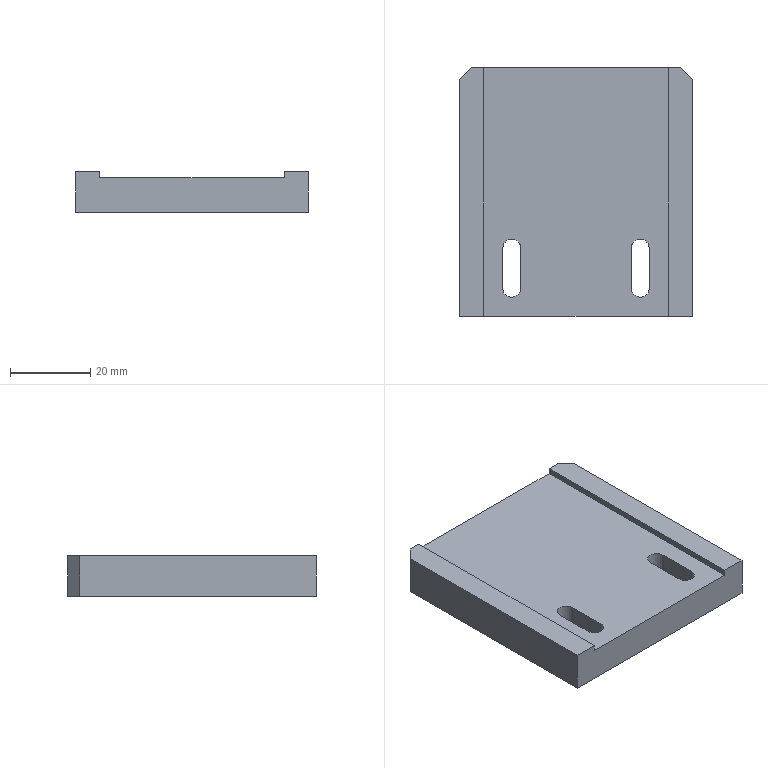Part | SolidWorks | features ICE 2, Chamfer 1, Extrusion 1, MirrorPattern 1 | 1 solid | 20 faces | box 58 x 62 x 10 mm | volume 30557 mm3 | plane 16 | cylinder 4 | commonest cylinder face diameters 4.5 x4
STEP:
#1=CARTESIAN_POINT('',(-18.25,-24.,0.));
#2=VERTEX_POINT('',#1);
#3=CARTESIAN_POINT('',(-13.75,-24.,0.));
#4=VERTEX_POINT('',#3);
#5=CARTESIAN_POINT('',(-16.,-24.,0.));
#6=DIRECTION('',(0.,0.,1.));
#7=DIRECTION('',(-1.,0.,0.));
#8=AXIS2_PLACEMENT_3D('',#5,#6,#7);
#9=CIRCLE('',#8,2.25);
#10=EDGE_CURVE('',#2,#4,#9,.T.);
#11=ORIENTED_EDGE('',*,*,#10,.T.);
#12=CARTESIAN_POINT('',(-13.75,-14.,0.));
#13=VERTEX_POINT('',#12);
#14=CARTESIAN_POINT('',(-13.75,-24.,0.));
#15=DIRECTION('',(0.,1.,0.));
#16=VECTOR('',#15,1000.);
#17=LINE('',#14,#16);
#18=EDGE_CURVE('',#4,#13,#17,.T.);
#19=ORIENTED_EDGE('',*,*,#18,.T.);
#20=CARTESIAN_POINT('',(-18.25,-14.,0.));
#21=VERTEX_POINT('',#20);
#22=CARTESIAN_POINT('',(-16.,-14.,0.));
#23=DIRECTION('',(0.,0.,1.));
#24=DIRECTION('',(-1.,0.,0.));
#25=AXIS2_PLACEMENT_3D('',#22,#23,#24);
#26=CIRCLE('',#25,2.25);
#27=EDGE_CURVE('',#13,#21,#26,.T.);
#28=ORIENTED_EDGE('',*,*,#27,.T.);
#29=CARTESIAN_POINT('',(-18.25,-24.,0.));
#30=DIRECTION('',(0.,-1.,0.));
#31=VECTOR('',#30,1000.);
#32=LINE('',#29,#31);
#33=EDGE_CURVE('',#21,#2,#32,.T.);
#34=ORIENTED_EDGE('',*,*,#33,.T.);
#35=EDGE_LOOP('',(#11,#19,#28,#34));
#36=FACE_BOUND('',#35,.T.);
#37=CARTESIAN_POINT('',(-29.,28.,0.));
#38=VERTEX_POINT('',#37);
#39=CARTESIAN_POINT('',(-29.,-31.,0.));
#40=VERTEX_POINT('',#39);
#41=CARTESIAN_POINT('',(-29.,-31.,0.));
#42=DIRECTION('',(0.,-1.,0.));
#43=VECTOR('',#42,1000.);
#44=LINE('',#41,#43);
#45=EDGE_CURVE('',#38,#40,#44,.T.);
#46=ORIENTED_EDGE('',*,*,#45,.F.);
#47=CARTESIAN_POINT('',(-26.,31.,0.));
#48=VERTEX_POINT('',#47);
#49=CARTESIAN_POINT('',(-28.5,28.5,0.));
#50=DIRECTION('',(0.7071,0.7071,0.));
#51=VECTOR('',#50,1000.);
#52=LINE('',#49,#51);
#53=EDGE_CURVE('',#38,#48,#52,.T.);
#54=ORIENTED_EDGE('',*,*,#53,.T.);
#55=CARTESIAN_POINT('',(26.,31.,0.));
#56=VERTEX_POINT('',#55);
#57=CARTESIAN_POINT('',(-29.,31.,0.));
#58=DIRECTION('',(-1.,0.,0.));
#59=VECTOR('',#58,1000.);
#60=LINE('',#57,#59);
#61=EDGE_CURVE('',#56,#48,#60,.T.);
#62=ORIENTED_EDGE('',*,*,#61,.F.);
#63=CARTESIAN_POINT('',(29.,28.,0.));
#64=VERTEX_POINT('',#63);
#65=CARTESIAN_POINT('',(28.5,28.5,0.));
#66=DIRECTION('',(0.7071,-0.7071,0.));
#67=VECTOR('',#66,1000.);
#68=LINE('',#65,#67);
#69=EDGE_CURVE('',#56,#64,#68,.T.);
#70=ORIENTED_EDGE('',*,*,#69,.T.);
#71=CARTESIAN_POINT('',(29.,-31.,0.));
#72=VERTEX_POINT('',#71);
#73=CARTESIAN_POINT('',(29.,-31.,0.));
#74=DIRECTION('',(0.,1.,0.));
#75=VECTOR('',#74,1000.);
#76=LINE('',#73,#75);
#77=EDGE_CURVE('',#72,#64,#76,.T.);
#78=ORIENTED_EDGE('',*,*,#77,.F.);
#79=CARTESIAN_POINT('',(-29.,-31.,0.));
#80=DIRECTION('',(1.,0.,0.));
#81=VECTOR('',#80,1000.);
#82=LINE('',#79,#81);
#83=EDGE_CURVE('',#40,#72,#82,.T.);
#84=ORIENTED_EDGE('',*,*,#83,.F.);
#85=EDGE_LOOP('',(#46,#54,#62,#70,#78,#84));
#86=FACE_OUTER_BOUND('',#85,.T.);
#87=CARTESIAN_POINT('',(13.75,-24.,0.));
#88=VERTEX_POINT('',#87);
#89=CARTESIAN_POINT('',(13.75,-14.,0.));
#90=VERTEX_POINT('',#89);
#91=CARTESIAN_POINT('',(13.75,-24.,0.));
#92=DIRECTION('',(0.,1.,0.));
#93=VECTOR('',#92,1000.);
#94=LINE('',#91,#93);
#95=EDGE_CURVE('',#88,#90,#94,.T.);
#96=ORIENTED_EDGE('',*,*,#95,.F.);
#97=CARTESIAN_POINT('',(18.25,-24.,0.));
#98=VERTEX_POINT('',#97);
#99=CARTESIAN_POINT('',(16.,-24.,0.));
#100=DIRECTION('',(0.,0.,-1.));
#101=DIRECTION('',(-1.,0.,0.));
#102=AXIS2_PLACEMENT_3D('',#99,#100,#101);
#103=CIRCLE('',#102,2.25);
#104=EDGE_CURVE('',#98,#88,#103,.T.);
#105=ORIENTED_EDGE('',*,*,#104,.F.);
#106=CARTESIAN_POINT('',(18.25,-14.,0.));
#107=VERTEX_POINT('',#106);
#108=CARTESIAN_POINT('',(18.25,-24.,0.));
#109=DIRECTION('',(0.,-1.,0.));
#110=VECTOR('',#109,1000.);
#111=LINE('',#108,#110);
#112=EDGE_CURVE('',#107,#98,#111,.T.);
#113=ORIENTED_EDGE('',*,*,#112,.F.);
#114=CARTESIAN_POINT('',(16.,-14.,0.));
#115=DIRECTION('',(0.,0.,-1.));
#116=DIRECTION('',(-1.,0.,0.));
#117=AXIS2_PLACEMENT_3D('',#114,#115,#116);
#118=CIRCLE('',#117,2.25);
#119=EDGE_CURVE('',#90,#107,#118,.T.);
#120=ORIENTED_EDGE('',*,*,#119,.F.);
#121=EDGE_LOOP('',(#96,#105,#113,#120));
#122=FACE_BOUND('',#121,.T.);
#123=CARTESIAN_POINT('',(0.,0.,0.));
#124=DIRECTION('',(0.,0.,-1.));
#125=DIRECTION('',(-1.,0.,0.));
#126=AXIS2_PLACEMENT_3D('',#123,#124,#125);
#127=PLANE('',#126);
#128=ADVANCED_FACE('',(#36,#86,#122),#127,.T.);
#129=CARTESIAN_POINT('',(23.,-31.,8.5));
#130=VERTEX_POINT('',#129);
#131=CARTESIAN_POINT('',(23.,31.,8.5));
#132=VERTEX_POINT('',#131);
#133=CARTESIAN_POINT('',(23.,-31.,8.5));
#134=DIRECTION('',(0.,1.,0.));
#135=VECTOR('',#134,1000.);
#136=LINE('',#133,#135);
#137=EDGE_CURVE('',#130,#132,#136,.T.);
#138=ORIENTED_EDGE('',*,*,#137,.T.);
#139=CARTESIAN_POINT('',(-23.,31.,8.5));
#140=VERTEX_POINT('',#139);
#141=CARTESIAN_POINT('',(-23.,31.,8.5));
#142=DIRECTION('',(-1.,0.,0.));
#143=VECTOR('',#142,1000.);
#144=LINE('',#141,#143);
#145=EDGE_CURVE('',#132,#140,#144,.T.);
#146=ORIENTED_EDGE('',*,*,#145,.T.);
#147=CARTESIAN_POINT('',(-23.,-31.,8.5));
#148=VERTEX_POINT('',#147);
#149=CARTESIAN_POINT('',(-23.,-31.,8.5));
#150=DIRECTION('',(0.,-1.,0.));
#151=VECTOR('',#150,1000.);
#152=LINE('',#149,#151);
#153=EDGE_CURVE('',#140,#148,#152,.T.);
#154=ORIENTED_EDGE('',*,*,#153,.T.);
#155=CARTESIAN_POINT('',(-23.,-31.,8.5));
#156=DIRECTION('',(1.,0.,0.));
#157=VECTOR('',#156,1000.);
#158=LINE('',#155,#157);
#159=EDGE_CURVE('',#148,#130,#158,.T.);
#160=ORIENTED_EDGE('',*,*,#159,.T.);
#161=EDGE_LOOP('',(#138,#146,#154,#160));
#162=FACE_OUTER_BOUND('',#161,.T.);
#163=CARTESIAN_POINT('',(-13.75,-24.,8.5));
#164=VERTEX_POINT('',#163);
#165=CARTESIAN_POINT('',(-13.75,-14.,8.5));
#166=VERTEX_POINT('',#165);
#167=CARTESIAN_POINT('',(-13.75,-24.,8.5));
#168=DIRECTION('',(0.,1.,0.));
#169=VECTOR('',#168,1000.);
#170=LINE('',#167,#169);
#171=EDGE_CURVE('',#164,#166,#170,.T.);
#172=ORIENTED_EDGE('',*,*,#171,.F.);
#173=CARTESIAN_POINT('',(-18.25,-24.,8.5));
#174=VERTEX_POINT('',#173);
#175=CARTESIAN_POINT('',(-16.,-24.,8.5));
#176=DIRECTION('',(0.,0.,1.));
#177=DIRECTION('',(1.,0.,0.));
#178=AXIS2_PLACEMENT_3D('',#175,#176,#177);
#179=CIRCLE('',#178,2.25);
#180=EDGE_CURVE('',#174,#164,#179,.T.);
#181=ORIENTED_EDGE('',*,*,#180,.F.);
#182=CARTESIAN_POINT('',(-18.25,-14.,8.5));
#183=VERTEX_POINT('',#182);
#184=CARTESIAN_POINT('',(-18.25,-24.,8.5));
#185=DIRECTION('',(0.,-1.,0.));
#186=VECTOR('',#185,1000.);
#187=LINE('',#184,#186);
#188=EDGE_CURVE('',#183,#174,#187,.T.);
#189=ORIENTED_EDGE('',*,*,#188,.F.);
#190=CARTESIAN_POINT('',(-16.,-14.,8.5));
#191=DIRECTION('',(0.,0.,1.));
#192=DIRECTION('',(1.,0.,0.));
#193=AXIS2_PLACEMENT_3D('',#190,#191,#192);
#194=CIRCLE('',#193,2.25);
#195=EDGE_CURVE('',#166,#183,#194,.T.);
#196=ORIENTED_EDGE('',*,*,#195,.F.);
#197=EDGE_LOOP('',(#172,#181,#189,#196));
#198=FACE_BOUND('',#197,.T.);
#199=CARTESIAN_POINT('',(18.25,-24.,8.5));
#200=VERTEX_POINT('',#199);
#201=CARTESIAN_POINT('',(13.75,-24.,8.5));
#202=VERTEX_POINT('',#201);
#203=CARTESIAN_POINT('',(16.,-24.,8.5));
#204=DIRECTION('',(0.,0.,-1.));
#205=DIRECTION('',(-1.,0.,0.));
#206=AXIS2_PLACEMENT_3D('',#203,#204,#205);
#207=CIRCLE('',#206,2.25);
#208=EDGE_CURVE('',#200,#202,#207,.T.);
#209=ORIENTED_EDGE('',*,*,#208,.T.);
#210=CARTESIAN_POINT('',(13.75,-14.,8.5));
#211=VERTEX_POINT('',#210);
#212=CARTESIAN_POINT('',(13.75,-24.,8.5));
#213=DIRECTION('',(0.,1.,0.));
#214=VECTOR('',#213,1000.);
#215=LINE('',#212,#214);
#216=EDGE_CURVE('',#202,#211,#215,.T.);
#217=ORIENTED_EDGE('',*,*,#216,.T.);
#218=CARTESIAN_POINT('',(18.25,-14.,8.5));
#219=VERTEX_POINT('',#218);
#220=CARTESIAN_POINT('',(16.,-14.,8.5));
#221=DIRECTION('',(0.,0.,-1.));
#222=DIRECTION('',(-1.,0.,0.));
#223=AXIS2_PLACEMENT_3D('',#220,#221,#222);
#224=CIRCLE('',#223,2.25);
#225=EDGE_CURVE('',#211,#219,#224,.T.);
#226=ORIENTED_EDGE('',*,*,#225,.T.);
#227=CARTESIAN_POINT('',(18.25,-24.,8.5));
#228=DIRECTION('',(0.,-1.,0.));
#229=VECTOR('',#228,1000.);
#230=LINE('',#227,#229);
#231=EDGE_CURVE('',#219,#200,#230,.T.);
#232=ORIENTED_EDGE('',*,*,#231,.T.);
#233=EDGE_LOOP('',(#209,#217,#226,#232));
#234=FACE_BOUND('',#233,.T.);
#235=CARTESIAN_POINT('',(0.,0.,8.5));
#236=DIRECTION('',(0.,0.,-1.));
#237=DIRECTION('',(-1.,0.,0.));
#238=AXIS2_PLACEMENT_3D('',#235,#236,#237);
#239=PLANE('',#238);
#240=ADVANCED_FACE('',(#162,#198,#234),#239,.F.);
#241=CARTESIAN_POINT('',(29.,-31.,10.));
#242=VERTEX_POINT('',#241);
#243=CARTESIAN_POINT('',(29.,28.,10.));
#244=VERTEX_POINT('',#243);
#245=CARTESIAN_POINT('',(29.,-31.,10.));
#246=DIRECTION('',(0.,1.,0.));
#247=VECTOR('',#246,1000.);
#248=LINE('',#245,#247);
#249=EDGE_CURVE('',#242,#244,#248,.T.);
#250=ORIENTED_EDGE('',*,*,#249,.T.);
#251=CARTESIAN_POINT('',(26.,31.,10.));
#252=VERTEX_POINT('',#251);
#253=CARTESIAN_POINT('',(26.,31.,10.));
#254=DIRECTION('',(-0.7071,0.7071,0.));
#255=VECTOR('',#254,1000.);
#256=LINE('',#253,#255);
#257=EDGE_CURVE('',#244,#252,#256,.T.);
#258=ORIENTED_EDGE('',*,*,#257,.T.);
#259=CARTESIAN_POINT('',(23.,31.,10.));
#260=VERTEX_POINT('',#259);
#261=CARTESIAN_POINT('',(-29.,31.,10.));
#262=DIRECTION('',(-1.,0.,0.));
#263=VECTOR('',#262,1000.);
#264=LINE('',#261,#263);
#265=EDGE_CURVE('',#252,#260,#264,.T.);
#266=ORIENTED_EDGE('',*,*,#265,.T.);
#267=CARTESIAN_POINT('',(23.,-31.,10.));
#268=VERTEX_POINT('',#267);
#269=CARTESIAN_POINT('',(23.,-31.,10.));
#270=DIRECTION('',(0.,1.,0.));
#271=VECTOR('',#270,1000.);
#272=LINE('',#269,#271);
#273=EDGE_CURVE('',#268,#260,#272,.T.);
#274=ORIENTED_EDGE('',*,*,#273,.F.);
#275=CARTESIAN_POINT('',(-29.,-31.,10.));
#276=DIRECTION('',(1.,0.,0.));
#277=VECTOR('',#276,1000.);
#278=LINE('',#275,#277);
#279=EDGE_CURVE('',#268,#242,#278,.T.);
#280=ORIENTED_EDGE('',*,*,#279,.T.);
#281=EDGE_LOOP('',(#250,#258,#266,#274,#280));
#282=FACE_OUTER_BOUND('',#281,.T.);
#283=CARTESIAN_POINT('',(0.,0.,10.));
#284=DIRECTION('',(0.,0.,-1.));
#285=DIRECTION('',(-1.,0.,0.));
#286=AXIS2_PLACEMENT_3D('',#283,#284,#285);
#287=PLANE('',#286);
#288=ADVANCED_FACE('',(#282),#287,.F.);
#289=ORIENTED_EDGE('',*,*,#77,.T.);
#290=CARTESIAN_POINT('',(29.,28.,10.));
#291=DIRECTION('',(0.,0.,1.));
#292=VECTOR('',#291,1000.);
#293=LINE('',#290,#292);
#294=EDGE_CURVE('',#64,#244,#293,.T.);
#295=ORIENTED_EDGE('',*,*,#294,.T.);
#296=ORIENTED_EDGE('',*,*,#249,.F.);
#297=CARTESIAN_POINT('',(29.,-31.,10.));
#298=DIRECTION('',(0.,0.,-1.));
#299=VECTOR('',#298,1000.);
#300=LINE('',#297,#299);
#301=EDGE_CURVE('',#242,#72,#300,.T.);
#302=ORIENTED_EDGE('',*,*,#301,.T.);
#303=EDGE_LOOP('',(#289,#295,#296,#302));
#304=FACE_OUTER_BOUND('',#303,.T.);
#305=CARTESIAN_POINT('',(29.,-31.,10.));
#306=DIRECTION('',(-1.,0.,0.));
#307=DIRECTION('',(0.,0.,1.));
#308=AXIS2_PLACEMENT_3D('',#305,#306,#307);
#309=PLANE('',#308);
#310=ADVANCED_FACE('',(#304),#309,.F.);
#311=ORIENTED_EDGE('',*,*,#61,.T.);
#312=CARTESIAN_POINT('',(-26.,31.,10.));
#313=VERTEX_POINT('',#312);
#314=CARTESIAN_POINT('',(-26.,31.,10.));
#315=DIRECTION('',(0.,0.,1.));
#316=VECTOR('',#315,1000.);
#317=LINE('',#314,#316);
#318=EDGE_CURVE('',#48,#313,#317,.T.);
#319=ORIENTED_EDGE('',*,*,#318,.T.);
#320=CARTESIAN_POINT('',(-23.,31.,10.));
#321=VERTEX_POINT('',#320);
#322=CARTESIAN_POINT('',(-29.,31.,10.));
#323=DIRECTION('',(-1.,0.,0.));
#324=VECTOR('',#323,1000.);
#325=LINE('',#322,#324);
#326=EDGE_CURVE('',#321,#313,#325,.T.);
#327=ORIENTED_EDGE('',*,*,#326,.F.);
#328=CARTESIAN_POINT('',(-23.,31.,8.5));
#329=DIRECTION('',(0.,0.,1.));
#330=VECTOR('',#329,1000.);
#331=LINE('',#328,#330);
#332=EDGE_CURVE('',#140,#321,#331,.T.);
#333=ORIENTED_EDGE('',*,*,#332,.F.);
#334=ORIENTED_EDGE('',*,*,#145,.F.);
#335=CARTESIAN_POINT('',(23.,31.,8.5));
#336=DIRECTION('',(0.,0.,1.));
#337=VECTOR('',#336,1000.);
#338=LINE('',#335,#337);
#339=EDGE_CURVE('',#132,#260,#338,.T.);
#340=ORIENTED_EDGE('',*,*,#339,.T.);
#341=ORIENTED_EDGE('',*,*,#265,.F.);
#342=CARTESIAN_POINT('',(26.,31.,10.));
#343=DIRECTION('',(0.,0.,-1.));
#344=VECTOR('',#343,1000.);
#345=LINE('',#342,#344);
#346=EDGE_CURVE('',#252,#56,#345,.T.);
#347=ORIENTED_EDGE('',*,*,#346,.T.);
#348=EDGE_LOOP('',(#311,#319,#327,#333,#334,#340,#341,#347));
#349=FACE_OUTER_BOUND('',#348,.T.);
#350=CARTESIAN_POINT('',(-29.,31.,10.));
#351=DIRECTION('',(0.,-1.,0.));
#352=DIRECTION('',(0.,0.,-1.));
#353=AXIS2_PLACEMENT_3D('',#350,#351,#352);
#354=PLANE('',#353);
#355=ADVANCED_FACE('',(#349),#354,.F.);
#356=CARTESIAN_POINT('',(-29.,28.,10.));
#357=VERTEX_POINT('',#356);
#358=CARTESIAN_POINT('',(-29.,-31.,10.));
#359=VERTEX_POINT('',#358);
#360=CARTESIAN_POINT('',(-29.,-31.,10.));
#361=DIRECTION('',(0.,-1.,0.));
#362=VECTOR('',#361,1000.);
#363=LINE('',#360,#362);
#364=EDGE_CURVE('',#357,#359,#363,.T.);
#365=ORIENTED_EDGE('',*,*,#364,.F.);
#366=CARTESIAN_POINT('',(-29.,28.,10.));
#367=DIRECTION('',(0.,0.,-1.));
#368=VECTOR('',#367,1000.);
#369=LINE('',#366,#368);
#370=EDGE_CURVE('',#357,#38,#369,.T.);
#371=ORIENTED_EDGE('',*,*,#370,.T.);
#372=ORIENTED_EDGE('',*,*,#45,.T.);
#373=CARTESIAN_POINT('',(-29.,-31.,10.));
#374=DIRECTION('',(0.,0.,-1.));
#375=VECTOR('',#374,1000.);
#376=LINE('',#373,#375);
#377=EDGE_CURVE('',#359,#40,#376,.T.);
#378=ORIENTED_EDGE('',*,*,#377,.F.);
#379=EDGE_LOOP('',(#365,#371,#372,#378));
#380=FACE_OUTER_BOUND('',#379,.T.);
#381=CARTESIAN_POINT('',(-29.,-31.,10.));
#382=DIRECTION('',(1.,0.,0.));
#383=DIRECTION('',(0.,0.,-1.));
#384=AXIS2_PLACEMENT_3D('',#381,#382,#383);
#385=PLANE('',#384);
#386=ADVANCED_FACE('',(#380),#385,.F.);
#387=ORIENTED_EDGE('',*,*,#279,.F.);
#388=CARTESIAN_POINT('',(23.,-31.,8.5));
#389=DIRECTION('',(0.,0.,1.));
#390=VECTOR('',#389,1000.);
#391=LINE('',#388,#390);
#392=EDGE_CURVE('',#130,#268,#391,.T.);
#393=ORIENTED_EDGE('',*,*,#392,.F.);
#394=ORIENTED_EDGE('',*,*,#159,.F.);
#395=CARTESIAN_POINT('',(-23.,-31.,10.));
#396=VERTEX_POINT('',#395);
#397=CARTESIAN_POINT('',(-23.,-31.,8.5));
#398=DIRECTION('',(0.,0.,1.));
#399=VECTOR('',#398,1000.);
#400=LINE('',#397,#399);
#401=EDGE_CURVE('',#148,#396,#400,.T.);
#402=ORIENTED_EDGE('',*,*,#401,.T.);
#403=CARTESIAN_POINT('',(-29.,-31.,10.));
#404=DIRECTION('',(1.,0.,0.));
#405=VECTOR('',#404,1000.);
#406=LINE('',#403,#405);
#407=EDGE_CURVE('',#359,#396,#406,.T.);
#408=ORIENTED_EDGE('',*,*,#407,.F.);
#409=ORIENTED_EDGE('',*,*,#377,.T.);
#410=ORIENTED_EDGE('',*,*,#83,.T.);
#411=ORIENTED_EDGE('',*,*,#301,.F.);
#412=EDGE_LOOP('',(#387,#393,#394,#402,#408,#409,#410,#411));
#413=FACE_OUTER_BOUND('',#412,.T.);
#414=CARTESIAN_POINT('',(-29.,-31.,10.));
#415=DIRECTION('',(0.,1.,0.));
#416=DIRECTION('',(0.,0.,1.));
#417=AXIS2_PLACEMENT_3D('',#414,#415,#416);
#418=PLANE('',#417);
#419=ADVANCED_FACE('',(#413),#418,.F.);
#420=ORIENTED_EDGE('',*,*,#326,.T.);
#421=CARTESIAN_POINT('',(-29.,28.,10.));
#422=DIRECTION('',(-0.7071,-0.7071,0.));
#423=VECTOR('',#422,1000.);
#424=LINE('',#421,#423);
#425=EDGE_CURVE('',#313,#357,#424,.T.);
#426=ORIENTED_EDGE('',*,*,#425,.T.);
#427=ORIENTED_EDGE('',*,*,#364,.T.);
#428=ORIENTED_EDGE('',*,*,#407,.T.);
#429=CARTESIAN_POINT('',(-23.,-31.,10.));
#430=DIRECTION('',(0.,-1.,0.));
#431=VECTOR('',#430,1000.);
#432=LINE('',#429,#431);
#433=EDGE_CURVE('',#321,#396,#432,.T.);
#434=ORIENTED_EDGE('',*,*,#433,.F.);
#435=EDGE_LOOP('',(#420,#426,#427,#428,#434));
#436=FACE_OUTER_BOUND('',#435,.T.);
#437=CARTESIAN_POINT('',(0.,0.,10.));
#438=DIRECTION('',(0.,0.,-1.));
#439=DIRECTION('',(-1.,0.,0.));
#440=AXIS2_PLACEMENT_3D('',#437,#438,#439);
#441=PLANE('',#440);
#442=ADVANCED_FACE('',(#436),#441,.F.);
#443=ORIENTED_EDGE('',*,*,#273,.T.);
#444=ORIENTED_EDGE('',*,*,#339,.F.);
#445=ORIENTED_EDGE('',*,*,#137,.F.);
#446=ORIENTED_EDGE('',*,*,#392,.T.);
#447=EDGE_LOOP('',(#443,#444,#445,#446));
#448=FACE_OUTER_BOUND('',#447,.T.);
#449=CARTESIAN_POINT('',(23.,-31.,8.5));
#450=DIRECTION('',(1.,0.,0.));
#451=DIRECTION('',(0.,0.,-1.));
#452=AXIS2_PLACEMENT_3D('',#449,#450,#451);
#453=PLANE('',#452);
#454=ADVANCED_FACE('',(#448),#453,.F.);
#455=ORIENTED_EDGE('',*,*,#433,.T.);
#456=ORIENTED_EDGE('',*,*,#401,.F.);
#457=ORIENTED_EDGE('',*,*,#153,.F.);
#458=ORIENTED_EDGE('',*,*,#332,.T.);
#459=EDGE_LOOP('',(#455,#456,#457,#458));
#460=FACE_OUTER_BOUND('',#459,.T.);
#461=CARTESIAN_POINT('',(-23.,-31.,8.5));
#462=DIRECTION('',(-1.,0.,0.));
#463=DIRECTION('',(0.,0.,1.));
#464=AXIS2_PLACEMENT_3D('',#461,#462,#463);
#465=PLANE('',#464);
#466=ADVANCED_FACE('',(#460),#465,.F.);
#467=ORIENTED_EDGE('',*,*,#425,.F.);
#468=ORIENTED_EDGE('',*,*,#318,.F.);
#469=ORIENTED_EDGE('',*,*,#53,.F.);
#470=ORIENTED_EDGE('',*,*,#370,.F.);
#471=EDGE_LOOP('',(#467,#468,#469,#470));
#472=FACE_OUTER_BOUND('',#471,.T.);
#473=CARTESIAN_POINT('',(-29.,28.,10.));
#474=DIRECTION('',(0.7071,-0.7071,0.));
#475=DIRECTION('',(0.,0.,-1.));
#476=AXIS2_PLACEMENT_3D('',#473,#474,#475);
#477=PLANE('',#476);
#478=ADVANCED_FACE('',(#472),#477,.F.);
#479=ORIENTED_EDGE('',*,*,#257,.F.);
#480=ORIENTED_EDGE('',*,*,#294,.F.);
#481=ORIENTED_EDGE('',*,*,#69,.F.);
#482=ORIENTED_EDGE('',*,*,#346,.F.);
#483=EDGE_LOOP('',(#479,#480,#481,#482));
#484=FACE_OUTER_BOUND('',#483,.T.);
#485=CARTESIAN_POINT('',(26.,31.,10.));
#486=DIRECTION('',(-0.7071,-0.7071,0.));
#487=DIRECTION('',(0.,0.,-1.));
#488=AXIS2_PLACEMENT_3D('',#485,#486,#487);
#489=PLANE('',#488);
#490=ADVANCED_FACE('',(#484),#489,.F.);
#491=CARTESIAN_POINT('',(-18.25,-24.,-0.001));
#492=DIRECTION('',(0.,0.,1.));
#493=VECTOR('',#492,1000.);
#494=LINE('',#491,#493);
#495=EDGE_CURVE('',#2,#174,#494,.T.);
#496=ORIENTED_EDGE('',*,*,#495,.T.);
#497=ORIENTED_EDGE('',*,*,#180,.T.);
#498=CARTESIAN_POINT('',(-13.75,-24.,-0.001));
#499=DIRECTION('',(0.,0.,1.));
#500=VECTOR('',#499,1000.);
#501=LINE('',#498,#500);
#502=EDGE_CURVE('',#4,#164,#501,.T.);
#503=ORIENTED_EDGE('',*,*,#502,.F.);
#504=ORIENTED_EDGE('',*,*,#10,.F.);
#505=EDGE_LOOP('',(#496,#497,#503,#504));
#506=FACE_OUTER_BOUND('',#505,.T.);
#507=CARTESIAN_POINT('',(-16.,-24.,-0.001));
#508=DIRECTION('',(0.,0.,1.));
#509=DIRECTION('',(1.,0.,0.));
#510=AXIS2_PLACEMENT_3D('',#507,#508,#509);
#511=CYLINDRICAL_SURFACE('',#510,2.25);
#512=ADVANCED_FACE('',(#506),#511,.F.);
#513=CARTESIAN_POINT('',(-18.25,-14.,-0.001));
#514=DIRECTION('',(0.,0.,1.));
#515=VECTOR('',#514,1000.);
#516=LINE('',#513,#515);
#517=EDGE_CURVE('',#21,#183,#516,.T.);
#518=ORIENTED_EDGE('',*,*,#517,.T.);
#519=ORIENTED_EDGE('',*,*,#188,.T.);
#520=ORIENTED_EDGE('',*,*,#495,.F.);
#521=ORIENTED_EDGE('',*,*,#33,.F.);
#522=EDGE_LOOP('',(#518,#519,#520,#521));
#523=FACE_OUTER_BOUND('',#522,.T.);
#524=CARTESIAN_POINT('',(-18.25,-24.,-0.001));
#525=DIRECTION('',(-1.,0.,0.));
#526=DIRECTION('',(0.,-1.,0.));
#527=AXIS2_PLACEMENT_3D('',#524,#525,#526);
#528=PLANE('',#527);
#529=ADVANCED_FACE('',(#523),#528,.F.);
#530=CARTESIAN_POINT('',(-13.75,-14.,-0.001));
#531=DIRECTION('',(0.,0.,1.));
#532=VECTOR('',#531,1000.);
#533=LINE('',#530,#532);
#534=EDGE_CURVE('',#13,#166,#533,.T.);
#535=ORIENTED_EDGE('',*,*,#534,.T.);
#536=ORIENTED_EDGE('',*,*,#195,.T.);
#537=ORIENTED_EDGE('',*,*,#517,.F.);
#538=ORIENTED_EDGE('',*,*,#27,.F.);
#539=EDGE_LOOP('',(#535,#536,#537,#538));
#540=FACE_OUTER_BOUND('',#539,.T.);
#541=CARTESIAN_POINT('',(-16.,-14.,-0.001));
#542=DIRECTION('',(0.,0.,1.));
#543=DIRECTION('',(1.,0.,0.));
#544=AXIS2_PLACEMENT_3D('',#541,#542,#543);
#545=CYLINDRICAL_SURFACE('',#544,2.25);
#546=ADVANCED_FACE('',(#540),#545,.F.);
#547=ORIENTED_EDGE('',*,*,#502,.T.);
#548=ORIENTED_EDGE('',*,*,#171,.T.);
#549=ORIENTED_EDGE('',*,*,#534,.F.);
#550=ORIENTED_EDGE('',*,*,#18,.F.);
#551=EDGE_LOOP('',(#547,#548,#549,#550));
#552=FACE_OUTER_BOUND('',#551,.T.);
#553=CARTESIAN_POINT('',(-13.75,-24.,-0.001));
#554=DIRECTION('',(1.,0.,0.));
#555=DIRECTION('',(0.,1.,0.));
#556=AXIS2_PLACEMENT_3D('',#553,#554,#555);
#557=PLANE('',#556);
#558=ADVANCED_FACE('',(#552),#557,.F.);
#559=ORIENTED_EDGE('',*,*,#104,.T.);
#560=CARTESIAN_POINT('',(13.75,-24.,-0.001));
#561=DIRECTION('',(0.,0.,1.));
#562=VECTOR('',#561,1000.);
#563=LINE('',#560,#562);
#564=EDGE_CURVE('',#88,#202,#563,.T.);
#565=ORIENTED_EDGE('',*,*,#564,.T.);
#566=ORIENTED_EDGE('',*,*,#208,.F.);
#567=CARTESIAN_POINT('',(18.25,-24.,-0.001));
#568=DIRECTION('',(0.,0.,1.));
#569=VECTOR('',#568,1000.);
#570=LINE('',#567,#569);
#571=EDGE_CURVE('',#98,#200,#570,.T.);
#572=ORIENTED_EDGE('',*,*,#571,.F.);
#573=EDGE_LOOP('',(#559,#565,#566,#572));
#574=FACE_OUTER_BOUND('',#573,.T.);
#575=CARTESIAN_POINT('',(16.,-24.,-0.001));
#576=DIRECTION('',(0.,0.,1.));
#577=DIRECTION('',(1.,0.,0.));
#578=AXIS2_PLACEMENT_3D('',#575,#576,#577);
#579=CYLINDRICAL_SURFACE('',#578,2.25);
#580=ADVANCED_FACE('',(#574),#579,.F.);
#581=ORIENTED_EDGE('',*,*,#95,.T.);
#582=CARTESIAN_POINT('',(13.75,-14.,-0.001));
#583=DIRECTION('',(0.,0.,1.));
#584=VECTOR('',#583,1000.);
#585=LINE('',#582,#584);
#586=EDGE_CURVE('',#90,#211,#585,.T.);
#587=ORIENTED_EDGE('',*,*,#586,.T.);
#588=ORIENTED_EDGE('',*,*,#216,.F.);
#589=ORIENTED_EDGE('',*,*,#564,.F.);
#590=EDGE_LOOP('',(#581,#587,#588,#589));
#591=FACE_OUTER_BOUND('',#590,.T.);
#592=CARTESIAN_POINT('',(13.75,-24.,-0.001));
#593=DIRECTION('',(1.,0.,0.));
#594=DIRECTION('',(0.,1.,0.));
#595=AXIS2_PLACEMENT_3D('',#592,#593,#594);
#596=PLANE('',#595);
#597=ADVANCED_FACE('',(#591),#596,.T.);
#598=ORIENTED_EDGE('',*,*,#119,.T.);
#599=CARTESIAN_POINT('',(18.25,-14.,-0.001));
#600=DIRECTION('',(0.,0.,1.));
#601=VECTOR('',#600,1000.);
#602=LINE('',#599,#601);
#603=EDGE_CURVE('',#107,#219,#602,.T.);
#604=ORIENTED_EDGE('',*,*,#603,.T.);
#605=ORIENTED_EDGE('',*,*,#225,.F.);
#606=ORIENTED_EDGE('',*,*,#586,.F.);
#607=EDGE_LOOP('',(#598,#604,#605,#606));
#608=FACE_OUTER_BOUND('',#607,.T.);
#609=CARTESIAN_POINT('',(16.,-14.,-0.001));
#610=DIRECTION('',(0.,0.,1.));
#611=DIRECTION('',(1.,0.,0.));
#612=AXIS2_PLACEMENT_3D('',#609,#610,#611);
#613=CYLINDRICAL_SURFACE('',#612,2.25);
#614=ADVANCED_FACE('',(#608),#613,.F.);
#615=ORIENTED_EDGE('',*,*,#112,.T.);
#616=ORIENTED_EDGE('',*,*,#571,.T.);
#617=ORIENTED_EDGE('',*,*,#231,.F.);
#618=ORIENTED_EDGE('',*,*,#603,.F.);
#619=EDGE_LOOP('',(#615,#616,#617,#618));
#620=FACE_OUTER_BOUND('',#619,.T.);
#621=CARTESIAN_POINT('',(18.25,-24.,-0.001));
#622=DIRECTION('',(-1.,0.,0.));
#623=DIRECTION('',(0.,-1.,0.));
#624=AXIS2_PLACEMENT_3D('',#621,#622,#623);
#625=PLANE('',#624);
#626=ADVANCED_FACE('',(#620),#625,.T.);
#627=CLOSED_SHELL('',(#128,#240,#288,#310,#355,#386,#419,#442,#454,#466,#478,#490,#512,#529,#546,#558,#580,#597,#614,#626));
#628=MANIFOLD_SOLID_BREP('',#627);
#629=CARTESIAN_POINT('',(0.,0.,0.));
#630=DIRECTION('',(0.,0.,1.));
#631=DIRECTION('',(1.,0.,0.));
#632=AXIS2_PLACEMENT_3D('',#629,#630,#631);
#633=(LENGTH_UNIT()NAMED_UNIT(*)SI_UNIT(.MILLI.,.METRE.));
#634=UNCERTAINTY_MEASURE_WITH_UNIT(LENGTH_MEASURE(0.00001),#633,'','');
#635=(NAMED_UNIT(*)PLANE_ANGLE_UNIT()SI_UNIT($,.RADIAN.));
#636=(NAMED_UNIT(*)SI_UNIT($,.STERADIAN.)SOLID_ANGLE_UNIT());
#637=(GEOMETRIC_REPRESENTATION_CONTEXT(3)GLOBAL_UNCERTAINTY_ASSIGNED_CONTEXT((#634))GLOBAL_UNIT_ASSIGNED_CONTEXT((#633,#635,#636))REPRESENTATION_CONTEXT('',''));
#638=ADVANCED_BREP_SHAPE_REPRESENTATION('',(#628,#632),#637);